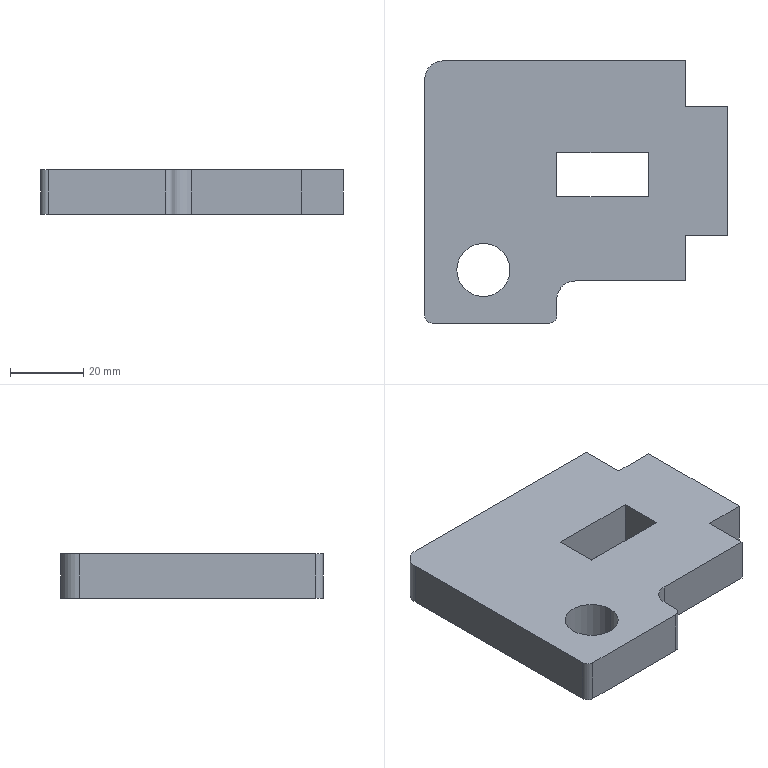Part | SolidWorks | features FlatPattern 1, SMBaseFlange 1, SheetMetal 1 | 1 solid | 22 faces | box 82.5 x 71.502 x 12 mm | volume 55316 mm3 | plane 16 | cylinder 6 | commonest cylinder face diameters 4 x2 10 x2 14.5 x2
STEP:
#1=CARTESIAN_POINT('',(-23.25,15.,12.));
#2=VERTEX_POINT('',#1);
#3=CARTESIAN_POINT('',(-8.75,15.,12.));
#4=VERTEX_POINT('',#3);
#5=CARTESIAN_POINT('',(-16.,15.,12.));
#6=DIRECTION('',(0.,0.,1.));
#7=DIRECTION('',(1.,0.,0.));
#8=AXIS2_PLACEMENT_3D('',#5,#6,#7);
#9=CIRCLE('',#8,7.25);
#10=EDGE_CURVE('',#2,#4,#9,.T.);
#11=ORIENTED_EDGE('',*,*,#10,.T.);
#12=CARTESIAN_POINT('',(-8.75,15.,0.));
#13=VERTEX_POINT('',#12);
#14=CARTESIAN_POINT('',(-8.75,15.,12.));
#15=DIRECTION('',(0.,0.,-1.));
#16=VECTOR('',#15,1000.);
#17=LINE('',#14,#16);
#18=EDGE_CURVE('',#4,#13,#17,.T.);
#19=ORIENTED_EDGE('',*,*,#18,.T.);
#20=CARTESIAN_POINT('',(-23.25,15.,0.));
#21=VERTEX_POINT('',#20);
#22=CARTESIAN_POINT('',(-16.,15.,0.));
#23=DIRECTION('',(0.,0.,1.));
#24=DIRECTION('',(1.,0.,0.));
#25=AXIS2_PLACEMENT_3D('',#22,#23,#24);
#26=CIRCLE('',#25,7.25);
#27=EDGE_CURVE('',#21,#13,#26,.T.);
#28=ORIENTED_EDGE('',*,*,#27,.F.);
#29=CARTESIAN_POINT('',(-23.25,15.,12.));
#30=DIRECTION('',(0.,0.,-1.));
#31=VECTOR('',#30,1000.);
#32=LINE('',#29,#31);
#33=EDGE_CURVE('',#2,#21,#32,.T.);
#34=ORIENTED_EDGE('',*,*,#33,.F.);
#35=EDGE_LOOP('',(#11,#19,#28,#34));
#36=FACE_OUTER_BOUND('',#35,.T.);
#37=CARTESIAN_POINT('',(-16.,15.,12.));
#38=DIRECTION('',(0.,0.,-1.));
#39=DIRECTION('',(-1.,0.,0.));
#40=AXIS2_PLACEMENT_3D('',#37,#38,#39);
#41=CYLINDRICAL_SURFACE('',#40,7.25);
#42=ADVANCED_FACE('',(#36),#41,.F.);
#43=CARTESIAN_POINT('',(39.,59.502,12.));
#44=VERTEX_POINT('',#43);
#45=CARTESIAN_POINT('',(39.,72.002,12.));
#46=VERTEX_POINT('',#45);
#47=CARTESIAN_POINT('',(39.,72.002,12.));
#48=DIRECTION('',(0.,1.,0.));
#49=VECTOR('',#48,1000.);
#50=LINE('',#47,#49);
#51=EDGE_CURVE('',#44,#46,#50,.T.);
#52=ORIENTED_EDGE('',*,*,#51,.T.);
#53=CARTESIAN_POINT('',(-27.,72.002,12.));
#54=VERTEX_POINT('',#53);
#55=CARTESIAN_POINT('',(-27.,72.002,12.));
#56=DIRECTION('',(-1.,0.,0.));
#57=VECTOR('',#56,1000.);
#58=LINE('',#55,#57);
#59=EDGE_CURVE('',#46,#54,#58,.T.);
#60=ORIENTED_EDGE('',*,*,#59,.T.);
#61=CARTESIAN_POINT('',(-32.,67.002,12.));
#62=VERTEX_POINT('',#61);
#63=CARTESIAN_POINT('',(-27.,67.002,12.));
#64=DIRECTION('',(0.,0.,1.));
#65=DIRECTION('',(-1.,0.,0.));
#66=AXIS2_PLACEMENT_3D('',#63,#64,#65);
#67=CIRCLE('',#66,5.);
#68=EDGE_CURVE('',#54,#62,#67,.T.);
#69=ORIENTED_EDGE('',*,*,#68,.T.);
#70=CARTESIAN_POINT('',(-32.,2.5,12.));
#71=VERTEX_POINT('',#70);
#72=CARTESIAN_POINT('',(-32.,2.5,12.));
#73=DIRECTION('',(0.,-1.,0.));
#74=VECTOR('',#73,1000.);
#75=LINE('',#72,#74);
#76=EDGE_CURVE('',#62,#71,#75,.T.);
#77=ORIENTED_EDGE('',*,*,#76,.T.);
#78=CARTESIAN_POINT('',(-30.,0.5,12.));
#79=VERTEX_POINT('',#78);
#80=CARTESIAN_POINT('',(-30.,2.5,12.));
#81=DIRECTION('',(0.,0.,1.));
#82=DIRECTION('',(-1.,0.,0.));
#83=AXIS2_PLACEMENT_3D('',#80,#81,#82);
#84=CIRCLE('',#83,2.);
#85=EDGE_CURVE('',#71,#79,#84,.T.);
#86=ORIENTED_EDGE('',*,*,#85,.T.);
#87=CARTESIAN_POINT('',(2.,0.5,12.));
#88=VERTEX_POINT('',#87);
#89=CARTESIAN_POINT('',(2.,0.5,12.));
#90=DIRECTION('',(1.,0.,0.));
#91=VECTOR('',#90,1000.);
#92=LINE('',#89,#91);
#93=EDGE_CURVE('',#79,#88,#92,.T.);
#94=ORIENTED_EDGE('',*,*,#93,.T.);
#95=CARTESIAN_POINT('',(4.,2.5,12.));
#96=VERTEX_POINT('',#95);
#97=CARTESIAN_POINT('',(2.,2.5,12.));
#98=DIRECTION('',(0.,0.,1.));
#99=DIRECTION('',(1.,0.,0.));
#100=AXIS2_PLACEMENT_3D('',#97,#98,#99);
#101=CIRCLE('',#100,2.);
#102=EDGE_CURVE('',#88,#96,#101,.T.);
#103=ORIENTED_EDGE('',*,*,#102,.T.);
#104=CARTESIAN_POINT('',(4.,7.002,12.));
#105=VERTEX_POINT('',#104);
#106=CARTESIAN_POINT('',(4.,7.002,12.));
#107=DIRECTION('',(0.,1.,0.));
#108=VECTOR('',#107,1000.);
#109=LINE('',#106,#108);
#110=EDGE_CURVE('',#96,#105,#109,.T.);
#111=ORIENTED_EDGE('',*,*,#110,.T.);
#112=CARTESIAN_POINT('',(9.,12.002,12.));
#113=VERTEX_POINT('',#112);
#114=CARTESIAN_POINT('',(9.,7.002,12.));
#115=DIRECTION('',(0.,0.,-1.));
#116=DIRECTION('',(1.,0.,0.));
#117=AXIS2_PLACEMENT_3D('',#114,#115,#116);
#118=CIRCLE('',#117,5.);
#119=EDGE_CURVE('',#105,#113,#118,.T.);
#120=ORIENTED_EDGE('',*,*,#119,.T.);
#121=CARTESIAN_POINT('',(39.,12.002,12.));
#122=VERTEX_POINT('',#121);
#123=CARTESIAN_POINT('',(39.,12.002,12.));
#124=DIRECTION('',(1.,0.,0.));
#125=VECTOR('',#124,1000.);
#126=LINE('',#123,#125);
#127=EDGE_CURVE('',#113,#122,#126,.T.);
#128=ORIENTED_EDGE('',*,*,#127,.T.);
#129=CARTESIAN_POINT('',(39.,24.502,12.));
#130=VERTEX_POINT('',#129);
#131=CARTESIAN_POINT('',(39.,24.502,12.));
#132=DIRECTION('',(0.,1.,0.));
#133=VECTOR('',#132,1000.);
#134=LINE('',#131,#133);
#135=EDGE_CURVE('',#122,#130,#134,.T.);
#136=ORIENTED_EDGE('',*,*,#135,.T.);
#137=CARTESIAN_POINT('',(50.5,24.502,12.));
#138=VERTEX_POINT('',#137);
#139=CARTESIAN_POINT('',(39.,24.502,12.));
#140=DIRECTION('',(1.,0.,0.));
#141=VECTOR('',#140,1000.);
#142=LINE('',#139,#141);
#143=EDGE_CURVE('',#130,#138,#142,.T.);
#144=ORIENTED_EDGE('',*,*,#143,.T.);
#145=CARTESIAN_POINT('',(50.5,59.502,12.));
#146=VERTEX_POINT('',#145);
#147=CARTESIAN_POINT('',(50.5,24.502,12.));
#148=DIRECTION('',(0.,1.,0.));
#149=VECTOR('',#148,1000.);
#150=LINE('',#147,#149);
#151=EDGE_CURVE('',#138,#146,#150,.T.);
#152=ORIENTED_EDGE('',*,*,#151,.T.);
#153=CARTESIAN_POINT('',(50.5,59.502,12.));
#154=DIRECTION('',(-1.,0.,0.));
#155=VECTOR('',#154,1000.);
#156=LINE('',#153,#155);
#157=EDGE_CURVE('',#146,#44,#156,.T.);
#158=ORIENTED_EDGE('',*,*,#157,.T.);
#159=EDGE_LOOP('',(#52,#60,#69,#77,#86,#94,#103,#111,#120,#128,#136,#144,#152,#158));
#160=FACE_OUTER_BOUND('',#159,.T.);
#161=ORIENTED_EDGE('',*,*,#10,.F.);
#162=CARTESIAN_POINT('',(-16.,15.,12.));
#163=DIRECTION('',(0.,0.,1.));
#164=DIRECTION('',(1.,0.,0.));
#165=AXIS2_PLACEMENT_3D('',#162,#163,#164);
#166=CIRCLE('',#165,7.25);
#167=EDGE_CURVE('',#4,#2,#166,.T.);
#168=ORIENTED_EDGE('',*,*,#167,.F.);
#169=EDGE_LOOP('',(#161,#168));
#170=FACE_BOUND('',#169,.T.);
#171=CARTESIAN_POINT('',(4.,35.002,12.));
#172=VERTEX_POINT('',#171);
#173=CARTESIAN_POINT('',(29.,35.002,12.));
#174=VERTEX_POINT('',#173);
#175=CARTESIAN_POINT('',(4.,35.002,12.));
#176=DIRECTION('',(1.,0.,0.));
#177=VECTOR('',#176,1000.);
#178=LINE('',#175,#177);
#179=EDGE_CURVE('',#172,#174,#178,.T.);
#180=ORIENTED_EDGE('',*,*,#179,.F.);
#181=CARTESIAN_POINT('',(4.,47.002,12.));
#182=VERTEX_POINT('',#181);
#183=CARTESIAN_POINT('',(4.,35.002,12.));
#184=DIRECTION('',(0.,-1.,0.));
#185=VECTOR('',#184,1000.);
#186=LINE('',#183,#185);
#187=EDGE_CURVE('',#182,#172,#186,.T.);
#188=ORIENTED_EDGE('',*,*,#187,.F.);
#189=CARTESIAN_POINT('',(29.,47.002,12.));
#190=VERTEX_POINT('',#189);
#191=CARTESIAN_POINT('',(4.,47.002,12.));
#192=DIRECTION('',(-1.,0.,0.));
#193=VECTOR('',#192,1000.);
#194=LINE('',#191,#193);
#195=EDGE_CURVE('',#190,#182,#194,.T.);
#196=ORIENTED_EDGE('',*,*,#195,.F.);
#197=CARTESIAN_POINT('',(29.,35.002,12.));
#198=DIRECTION('',(0.,1.,0.));
#199=VECTOR('',#198,1000.);
#200=LINE('',#197,#199);
#201=EDGE_CURVE('',#174,#190,#200,.T.);
#202=ORIENTED_EDGE('',*,*,#201,.F.);
#203=EDGE_LOOP('',(#180,#188,#196,#202));
#204=FACE_BOUND('',#203,.T.);
#205=CARTESIAN_POINT('',(9.,7.002,12.));
#206=DIRECTION('',(0.,0.,1.));
#207=DIRECTION('',(1.,0.,0.));
#208=AXIS2_PLACEMENT_3D('',#205,#206,#207);
#209=PLANE('',#208);
#210=ADVANCED_FACE('',(#160,#170,#204),#209,.T.);
#211=ORIENTED_EDGE('',*,*,#27,.T.);
#212=CARTESIAN_POINT('',(-16.,15.,0.));
#213=DIRECTION('',(0.,0.,1.));
#214=DIRECTION('',(1.,0.,0.));
#215=AXIS2_PLACEMENT_3D('',#212,#213,#214);
#216=CIRCLE('',#215,7.25);
#217=EDGE_CURVE('',#13,#21,#216,.T.);
#218=ORIENTED_EDGE('',*,*,#217,.T.);
#219=EDGE_LOOP('',(#211,#218));
#220=FACE_BOUND('',#219,.T.);
#221=CARTESIAN_POINT('',(39.,59.502,0.));
#222=VERTEX_POINT('',#221);
#223=CARTESIAN_POINT('',(39.,72.002,0.));
#224=VERTEX_POINT('',#223);
#225=CARTESIAN_POINT('',(39.,72.002,0.));
#226=DIRECTION('',(0.,1.,0.));
#227=VECTOR('',#226,1000.);
#228=LINE('',#225,#227);
#229=EDGE_CURVE('',#222,#224,#228,.T.);
#230=ORIENTED_EDGE('',*,*,#229,.F.);
#231=CARTESIAN_POINT('',(50.5,59.502,0.));
#232=VERTEX_POINT('',#231);
#233=CARTESIAN_POINT('',(50.5,59.502,0.));
#234=DIRECTION('',(-1.,0.,0.));
#235=VECTOR('',#234,1000.);
#236=LINE('',#233,#235);
#237=EDGE_CURVE('',#232,#222,#236,.T.);
#238=ORIENTED_EDGE('',*,*,#237,.F.);
#239=CARTESIAN_POINT('',(50.5,24.502,0.));
#240=VERTEX_POINT('',#239);
#241=CARTESIAN_POINT('',(50.5,24.502,0.));
#242=DIRECTION('',(0.,1.,0.));
#243=VECTOR('',#242,1000.);
#244=LINE('',#241,#243);
#245=EDGE_CURVE('',#240,#232,#244,.T.);
#246=ORIENTED_EDGE('',*,*,#245,.F.);
#247=CARTESIAN_POINT('',(39.,24.502,0.));
#248=VERTEX_POINT('',#247);
#249=CARTESIAN_POINT('',(39.,24.502,0.));
#250=DIRECTION('',(1.,0.,0.));
#251=VECTOR('',#250,1000.);
#252=LINE('',#249,#251);
#253=EDGE_CURVE('',#248,#240,#252,.T.);
#254=ORIENTED_EDGE('',*,*,#253,.F.);
#255=CARTESIAN_POINT('',(39.,12.002,0.));
#256=VERTEX_POINT('',#255);
#257=CARTESIAN_POINT('',(39.,24.502,0.));
#258=DIRECTION('',(0.,1.,0.));
#259=VECTOR('',#258,1000.);
#260=LINE('',#257,#259);
#261=EDGE_CURVE('',#256,#248,#260,.T.);
#262=ORIENTED_EDGE('',*,*,#261,.F.);
#263=CARTESIAN_POINT('',(9.,12.002,0.));
#264=VERTEX_POINT('',#263);
#265=CARTESIAN_POINT('',(39.,12.002,0.));
#266=DIRECTION('',(1.,0.,0.));
#267=VECTOR('',#266,1000.);
#268=LINE('',#265,#267);
#269=EDGE_CURVE('',#264,#256,#268,.T.);
#270=ORIENTED_EDGE('',*,*,#269,.F.);
#271=CARTESIAN_POINT('',(4.,7.002,0.));
#272=VERTEX_POINT('',#271);
#273=CARTESIAN_POINT('',(9.,7.002,0.));
#274=DIRECTION('',(0.,0.,-1.));
#275=DIRECTION('',(1.,0.,0.));
#276=AXIS2_PLACEMENT_3D('',#273,#274,#275);
#277=CIRCLE('',#276,5.);
#278=EDGE_CURVE('',#272,#264,#277,.T.);
#279=ORIENTED_EDGE('',*,*,#278,.F.);
#280=CARTESIAN_POINT('',(4.,2.5,0.));
#281=VERTEX_POINT('',#280);
#282=CARTESIAN_POINT('',(4.,7.002,0.));
#283=DIRECTION('',(0.,1.,0.));
#284=VECTOR('',#283,1000.);
#285=LINE('',#282,#284);
#286=EDGE_CURVE('',#281,#272,#285,.T.);
#287=ORIENTED_EDGE('',*,*,#286,.F.);
#288=CARTESIAN_POINT('',(2.,0.5,0.));
#289=VERTEX_POINT('',#288);
#290=CARTESIAN_POINT('',(2.,2.5,0.));
#291=DIRECTION('',(0.,0.,1.));
#292=DIRECTION('',(1.,0.,0.));
#293=AXIS2_PLACEMENT_3D('',#290,#291,#292);
#294=CIRCLE('',#293,2.);
#295=EDGE_CURVE('',#289,#281,#294,.T.);
#296=ORIENTED_EDGE('',*,*,#295,.F.);
#297=CARTESIAN_POINT('',(-30.,0.5,0.));
#298=VERTEX_POINT('',#297);
#299=CARTESIAN_POINT('',(2.,0.5,0.));
#300=DIRECTION('',(1.,0.,0.));
#301=VECTOR('',#300,1000.);
#302=LINE('',#299,#301);
#303=EDGE_CURVE('',#298,#289,#302,.T.);
#304=ORIENTED_EDGE('',*,*,#303,.F.);
#305=CARTESIAN_POINT('',(-32.,2.5,0.));
#306=VERTEX_POINT('',#305);
#307=CARTESIAN_POINT('',(-30.,2.5,0.));
#308=DIRECTION('',(0.,0.,1.));
#309=DIRECTION('',(-1.,0.,0.));
#310=AXIS2_PLACEMENT_3D('',#307,#308,#309);
#311=CIRCLE('',#310,2.);
#312=EDGE_CURVE('',#306,#298,#311,.T.);
#313=ORIENTED_EDGE('',*,*,#312,.F.);
#314=CARTESIAN_POINT('',(-32.,67.002,0.));
#315=VERTEX_POINT('',#314);
#316=CARTESIAN_POINT('',(-32.,2.5,0.));
#317=DIRECTION('',(0.,-1.,0.));
#318=VECTOR('',#317,1000.);
#319=LINE('',#316,#318);
#320=EDGE_CURVE('',#315,#306,#319,.T.);
#321=ORIENTED_EDGE('',*,*,#320,.F.);
#322=CARTESIAN_POINT('',(-27.,72.002,0.));
#323=VERTEX_POINT('',#322);
#324=CARTESIAN_POINT('',(-27.,67.002,0.));
#325=DIRECTION('',(0.,0.,1.));
#326=DIRECTION('',(-1.,0.,0.));
#327=AXIS2_PLACEMENT_3D('',#324,#325,#326);
#328=CIRCLE('',#327,5.);
#329=EDGE_CURVE('',#323,#315,#328,.T.);
#330=ORIENTED_EDGE('',*,*,#329,.F.);
#331=CARTESIAN_POINT('',(-27.,72.002,0.));
#332=DIRECTION('',(-1.,0.,0.));
#333=VECTOR('',#332,1000.);
#334=LINE('',#331,#333);
#335=EDGE_CURVE('',#224,#323,#334,.T.);
#336=ORIENTED_EDGE('',*,*,#335,.F.);
#337=EDGE_LOOP('',(#230,#238,#246,#254,#262,#270,#279,#287,#296,#304,#313,#321,#330,#336));
#338=FACE_OUTER_BOUND('',#337,.T.);
#339=CARTESIAN_POINT('',(4.,47.002,0.));
#340=VERTEX_POINT('',#339);
#341=CARTESIAN_POINT('',(4.,35.002,0.));
#342=VERTEX_POINT('',#341);
#343=CARTESIAN_POINT('',(4.,35.002,0.));
#344=DIRECTION('',(0.,-1.,0.));
#345=VECTOR('',#344,1000.);
#346=LINE('',#343,#345);
#347=EDGE_CURVE('',#340,#342,#346,.T.);
#348=ORIENTED_EDGE('',*,*,#347,.T.);
#349=CARTESIAN_POINT('',(29.,35.002,0.));
#350=VERTEX_POINT('',#349);
#351=CARTESIAN_POINT('',(4.,35.002,0.));
#352=DIRECTION('',(1.,0.,0.));
#353=VECTOR('',#352,1000.);
#354=LINE('',#351,#353);
#355=EDGE_CURVE('',#342,#350,#354,.T.);
#356=ORIENTED_EDGE('',*,*,#355,.T.);
#357=CARTESIAN_POINT('',(29.,47.002,0.));
#358=VERTEX_POINT('',#357);
#359=CARTESIAN_POINT('',(29.,35.002,0.));
#360=DIRECTION('',(0.,1.,0.));
#361=VECTOR('',#360,1000.);
#362=LINE('',#359,#361);
#363=EDGE_CURVE('',#350,#358,#362,.T.);
#364=ORIENTED_EDGE('',*,*,#363,.T.);
#365=CARTESIAN_POINT('',(4.,47.002,0.));
#366=DIRECTION('',(-1.,0.,0.));
#367=VECTOR('',#366,1000.);
#368=LINE('',#365,#367);
#369=EDGE_CURVE('',#358,#340,#368,.T.);
#370=ORIENTED_EDGE('',*,*,#369,.T.);
#371=EDGE_LOOP('',(#348,#356,#364,#370));
#372=FACE_BOUND('',#371,.T.);
#373=CARTESIAN_POINT('',(9.,7.002,0.));
#374=DIRECTION('',(0.,0.,1.));
#375=DIRECTION('',(1.,0.,0.));
#376=AXIS2_PLACEMENT_3D('',#373,#374,#375);
#377=PLANE('',#376);
#378=ADVANCED_FACE('',(#220,#338,#372),#377,.F.);
#379=ORIENTED_EDGE('',*,*,#229,.T.);
#380=CARTESIAN_POINT('',(39.,72.002,12.));
#381=DIRECTION('',(0.,0.,-1.));
#382=VECTOR('',#381,1000.);
#383=LINE('',#380,#382);
#384=EDGE_CURVE('',#46,#224,#383,.T.);
#385=ORIENTED_EDGE('',*,*,#384,.F.);
#386=ORIENTED_EDGE('',*,*,#51,.F.);
#387=CARTESIAN_POINT('',(39.,59.502,12.));
#388=DIRECTION('',(0.,0.,-1.));
#389=VECTOR('',#388,1000.);
#390=LINE('',#387,#389);
#391=EDGE_CURVE('',#44,#222,#390,.T.);
#392=ORIENTED_EDGE('',*,*,#391,.T.);
#393=EDGE_LOOP('',(#379,#385,#386,#392));
#394=FACE_OUTER_BOUND('',#393,.T.);
#395=CARTESIAN_POINT('',(39.,72.002,12.));
#396=DIRECTION('',(-1.,0.,0.));
#397=DIRECTION('',(0.,0.,1.));
#398=AXIS2_PLACEMENT_3D('',#395,#396,#397);
#399=PLANE('',#398);
#400=ADVANCED_FACE('',(#394),#399,.F.);
#401=ORIENTED_EDGE('',*,*,#335,.T.);
#402=CARTESIAN_POINT('',(-27.,72.002,12.));
#403=DIRECTION('',(0.,0.,-1.));
#404=VECTOR('',#403,1000.);
#405=LINE('',#402,#404);
#406=EDGE_CURVE('',#54,#323,#405,.T.);
#407=ORIENTED_EDGE('',*,*,#406,.F.);
#408=ORIENTED_EDGE('',*,*,#59,.F.);
#409=ORIENTED_EDGE('',*,*,#384,.T.);
#410=EDGE_LOOP('',(#401,#407,#408,#409));
#411=FACE_OUTER_BOUND('',#410,.T.);
#412=CARTESIAN_POINT('',(-27.,72.002,12.));
#413=DIRECTION('',(0.,-1.,0.));
#414=DIRECTION('',(0.,0.,-1.));
#415=AXIS2_PLACEMENT_3D('',#412,#413,#414);
#416=PLANE('',#415);
#417=ADVANCED_FACE('',(#411),#416,.F.);
#418=ORIENTED_EDGE('',*,*,#329,.T.);
#419=CARTESIAN_POINT('',(-32.,67.002,12.));
#420=DIRECTION('',(0.,0.,-1.));
#421=VECTOR('',#420,1000.);
#422=LINE('',#419,#421);
#423=EDGE_CURVE('',#62,#315,#422,.T.);
#424=ORIENTED_EDGE('',*,*,#423,.F.);
#425=ORIENTED_EDGE('',*,*,#68,.F.);
#426=ORIENTED_EDGE('',*,*,#406,.T.);
#427=EDGE_LOOP('',(#418,#424,#425,#426));
#428=FACE_OUTER_BOUND('',#427,.T.);
#429=CARTESIAN_POINT('',(-27.,67.002,12.));
#430=DIRECTION('',(0.,0.,-1.));
#431=DIRECTION('',(-1.,0.,0.));
#432=AXIS2_PLACEMENT_3D('',#429,#430,#431);
#433=CYLINDRICAL_SURFACE('',#432,5.);
#434=ADVANCED_FACE('',(#428),#433,.T.);
#435=ORIENTED_EDGE('',*,*,#320,.T.);
#436=CARTESIAN_POINT('',(-32.,2.5,12.));
#437=DIRECTION('',(0.,0.,-1.));
#438=VECTOR('',#437,1000.);
#439=LINE('',#436,#438);
#440=EDGE_CURVE('',#71,#306,#439,.T.);
#441=ORIENTED_EDGE('',*,*,#440,.F.);
#442=ORIENTED_EDGE('',*,*,#76,.F.);
#443=ORIENTED_EDGE('',*,*,#423,.T.);
#444=EDGE_LOOP('',(#435,#441,#442,#443));
#445=FACE_OUTER_BOUND('',#444,.T.);
#446=CARTESIAN_POINT('',(-32.,2.5,12.));
#447=DIRECTION('',(1.,0.,0.));
#448=DIRECTION('',(0.,1.,0.));
#449=AXIS2_PLACEMENT_3D('',#446,#447,#448);
#450=PLANE('',#449);
#451=ADVANCED_FACE('',(#445),#450,.F.);
#452=ORIENTED_EDGE('',*,*,#312,.T.);
#453=CARTESIAN_POINT('',(-30.,0.5,12.));
#454=DIRECTION('',(0.,0.,-1.));
#455=VECTOR('',#454,1000.);
#456=LINE('',#453,#455);
#457=EDGE_CURVE('',#79,#298,#456,.T.);
#458=ORIENTED_EDGE('',*,*,#457,.F.);
#459=ORIENTED_EDGE('',*,*,#85,.F.);
#460=ORIENTED_EDGE('',*,*,#440,.T.);
#461=EDGE_LOOP('',(#452,#458,#459,#460));
#462=FACE_OUTER_BOUND('',#461,.T.);
#463=CARTESIAN_POINT('',(-30.,2.5,12.));
#464=DIRECTION('',(0.,0.,-1.));
#465=DIRECTION('',(-1.,0.,0.));
#466=AXIS2_PLACEMENT_3D('',#463,#464,#465);
#467=CYLINDRICAL_SURFACE('',#466,2.);
#468=ADVANCED_FACE('',(#462),#467,.T.);
#469=ORIENTED_EDGE('',*,*,#303,.T.);
#470=CARTESIAN_POINT('',(2.,0.5,12.));
#471=DIRECTION('',(0.,0.,-1.));
#472=VECTOR('',#471,1000.);
#473=LINE('',#470,#472);
#474=EDGE_CURVE('',#88,#289,#473,.T.);
#475=ORIENTED_EDGE('',*,*,#474,.F.);
#476=ORIENTED_EDGE('',*,*,#93,.F.);
#477=ORIENTED_EDGE('',*,*,#457,.T.);
#478=EDGE_LOOP('',(#469,#475,#476,#477));
#479=FACE_OUTER_BOUND('',#478,.T.);
#480=CARTESIAN_POINT('',(2.,0.5,12.));
#481=DIRECTION('',(0.,1.,0.));
#482=DIRECTION('',(-1.,0.,0.));
#483=AXIS2_PLACEMENT_3D('',#480,#481,#482);
#484=PLANE('',#483);
#485=ADVANCED_FACE('',(#479),#484,.F.);
#486=ORIENTED_EDGE('',*,*,#295,.T.);
#487=CARTESIAN_POINT('',(4.,2.5,12.));
#488=DIRECTION('',(0.,0.,-1.));
#489=VECTOR('',#488,1000.);
#490=LINE('',#487,#489);
#491=EDGE_CURVE('',#96,#281,#490,.T.);
#492=ORIENTED_EDGE('',*,*,#491,.F.);
#493=ORIENTED_EDGE('',*,*,#102,.F.);
#494=ORIENTED_EDGE('',*,*,#474,.T.);
#495=EDGE_LOOP('',(#486,#492,#493,#494));
#496=FACE_OUTER_BOUND('',#495,.T.);
#497=CARTESIAN_POINT('',(2.,2.5,12.));
#498=DIRECTION('',(0.,0.,-1.));
#499=DIRECTION('',(-1.,0.,0.));
#500=AXIS2_PLACEMENT_3D('',#497,#498,#499);
#501=CYLINDRICAL_SURFACE('',#500,2.);
#502=ADVANCED_FACE('',(#496),#501,.T.);
#503=ORIENTED_EDGE('',*,*,#286,.T.);
#504=CARTESIAN_POINT('',(4.,7.002,12.));
#505=DIRECTION('',(0.,0.,-1.));
#506=VECTOR('',#505,1000.);
#507=LINE('',#504,#506);
#508=EDGE_CURVE('',#105,#272,#507,.T.);
#509=ORIENTED_EDGE('',*,*,#508,.F.);
#510=ORIENTED_EDGE('',*,*,#110,.F.);
#511=ORIENTED_EDGE('',*,*,#491,.T.);
#512=EDGE_LOOP('',(#503,#509,#510,#511));
#513=FACE_OUTER_BOUND('',#512,.T.);
#514=CARTESIAN_POINT('',(4.,7.002,12.));
#515=DIRECTION('',(-1.,0.,0.));
#516=DIRECTION('',(0.,0.,1.));
#517=AXIS2_PLACEMENT_3D('',#514,#515,#516);
#518=PLANE('',#517);
#519=ADVANCED_FACE('',(#513),#518,.F.);
#520=ORIENTED_EDGE('',*,*,#278,.T.);
#521=CARTESIAN_POINT('',(9.,12.002,12.));
#522=DIRECTION('',(0.,0.,-1.));
#523=VECTOR('',#522,1000.);
#524=LINE('',#521,#523);
#525=EDGE_CURVE('',#113,#264,#524,.T.);
#526=ORIENTED_EDGE('',*,*,#525,.F.);
#527=ORIENTED_EDGE('',*,*,#119,.F.);
#528=ORIENTED_EDGE('',*,*,#508,.T.);
#529=EDGE_LOOP('',(#520,#526,#527,#528));
#530=FACE_OUTER_BOUND('',#529,.T.);
#531=CARTESIAN_POINT('',(9.,7.002,12.));
#532=DIRECTION('',(0.,0.,-1.));
#533=DIRECTION('',(-1.,0.,0.));
#534=AXIS2_PLACEMENT_3D('',#531,#532,#533);
#535=CYLINDRICAL_SURFACE('',#534,5.);
#536=ADVANCED_FACE('',(#530),#535,.F.);
#537=ORIENTED_EDGE('',*,*,#269,.T.);
#538=CARTESIAN_POINT('',(39.,12.002,12.));
#539=DIRECTION('',(0.,0.,-1.));
#540=VECTOR('',#539,1000.);
#541=LINE('',#538,#540);
#542=EDGE_CURVE('',#122,#256,#541,.T.);
#543=ORIENTED_EDGE('',*,*,#542,.F.);
#544=ORIENTED_EDGE('',*,*,#127,.F.);
#545=ORIENTED_EDGE('',*,*,#525,.T.);
#546=EDGE_LOOP('',(#537,#543,#544,#545));
#547=FACE_OUTER_BOUND('',#546,.T.);
#548=CARTESIAN_POINT('',(39.,12.002,12.));
#549=DIRECTION('',(0.,1.,0.));
#550=DIRECTION('',(-1.,0.,0.));
#551=AXIS2_PLACEMENT_3D('',#548,#549,#550);
#552=PLANE('',#551);
#553=ADVANCED_FACE('',(#547),#552,.F.);
#554=ORIENTED_EDGE('',*,*,#261,.T.);
#555=CARTESIAN_POINT('',(39.,24.502,12.));
#556=DIRECTION('',(0.,0.,-1.));
#557=VECTOR('',#556,1000.);
#558=LINE('',#555,#557);
#559=EDGE_CURVE('',#130,#248,#558,.T.);
#560=ORIENTED_EDGE('',*,*,#559,.F.);
#561=ORIENTED_EDGE('',*,*,#135,.F.);
#562=ORIENTED_EDGE('',*,*,#542,.T.);
#563=EDGE_LOOP('',(#554,#560,#561,#562));
#564=FACE_OUTER_BOUND('',#563,.T.);
#565=CARTESIAN_POINT('',(39.,24.502,12.));
#566=DIRECTION('',(-1.,0.,0.));
#567=DIRECTION('',(0.,0.,1.));
#568=AXIS2_PLACEMENT_3D('',#565,#566,#567);
#569=PLANE('',#568);
#570=ADVANCED_FACE('',(#564),#569,.F.);
#571=ORIENTED_EDGE('',*,*,#253,.T.);
#572=CARTESIAN_POINT('',(50.5,24.502,12.));
#573=DIRECTION('',(0.,0.,-1.));
#574=VECTOR('',#573,1000.);
#575=LINE('',#572,#574);
#576=EDGE_CURVE('',#138,#240,#575,.T.);
#577=ORIENTED_EDGE('',*,*,#576,.F.);
#578=ORIENTED_EDGE('',*,*,#143,.F.);
#579=ORIENTED_EDGE('',*,*,#559,.T.);
#580=EDGE_LOOP('',(#571,#577,#578,#579));
#581=FACE_OUTER_BOUND('',#580,.T.);
#582=CARTESIAN_POINT('',(39.,24.502,12.));
#583=DIRECTION('',(0.,1.,0.));
#584=DIRECTION('',(0.,0.,1.));
#585=AXIS2_PLACEMENT_3D('',#582,#583,#584);
#586=PLANE('',#585);
#587=ADVANCED_FACE('',(#581),#586,.F.);
#588=ORIENTED_EDGE('',*,*,#245,.T.);
#589=CARTESIAN_POINT('',(50.5,59.502,12.));
#590=DIRECTION('',(0.,0.,-1.));
#591=VECTOR('',#590,1000.);
#592=LINE('',#589,#591);
#593=EDGE_CURVE('',#146,#232,#592,.T.);
#594=ORIENTED_EDGE('',*,*,#593,.F.);
#595=ORIENTED_EDGE('',*,*,#151,.F.);
#596=ORIENTED_EDGE('',*,*,#576,.T.);
#597=EDGE_LOOP('',(#588,#594,#595,#596));
#598=FACE_OUTER_BOUND('',#597,.T.);
#599=CARTESIAN_POINT('',(50.5,24.502,12.));
#600=DIRECTION('',(-1.,0.,0.));
#601=DIRECTION('',(0.,0.,1.));
#602=AXIS2_PLACEMENT_3D('',#599,#600,#601);
#603=PLANE('',#602);
#604=ADVANCED_FACE('',(#598),#603,.F.);
#605=ORIENTED_EDGE('',*,*,#237,.T.);
#606=ORIENTED_EDGE('',*,*,#391,.F.);
#607=ORIENTED_EDGE('',*,*,#157,.F.);
#608=ORIENTED_EDGE('',*,*,#593,.T.);
#609=EDGE_LOOP('',(#605,#606,#607,#608));
#610=FACE_OUTER_BOUND('',#609,.T.);
#611=CARTESIAN_POINT('',(50.5,59.502,12.));
#612=DIRECTION('',(0.,-1.,0.));
#613=DIRECTION('',(0.,0.,-1.));
#614=AXIS2_PLACEMENT_3D('',#611,#612,#613);
#615=PLANE('',#614);
#616=ADVANCED_FACE('',(#610),#615,.F.);
#617=ORIENTED_EDGE('',*,*,#18,.F.);
#618=ORIENTED_EDGE('',*,*,#167,.T.);
#619=ORIENTED_EDGE('',*,*,#33,.T.);
#620=ORIENTED_EDGE('',*,*,#217,.F.);
#621=EDGE_LOOP('',(#617,#618,#619,#620));
#622=FACE_OUTER_BOUND('',#621,.T.);
#623=CARTESIAN_POINT('',(-16.,15.,12.));
#624=DIRECTION('',(0.,0.,-1.));
#625=DIRECTION('',(-1.,0.,0.));
#626=AXIS2_PLACEMENT_3D('',#623,#624,#625);
#627=CYLINDRICAL_SURFACE('',#626,7.25);
#628=ADVANCED_FACE('',(#622),#627,.F.);
#629=ORIENTED_EDGE('',*,*,#347,.F.);
#630=CARTESIAN_POINT('',(4.,47.002,12.));
#631=DIRECTION('',(0.,0.,-1.));
#632=VECTOR('',#631,1000.);
#633=LINE('',#630,#632);
#634=EDGE_CURVE('',#182,#340,#633,.T.);
#635=ORIENTED_EDGE('',*,*,#634,.F.);
#636=ORIENTED_EDGE('',*,*,#187,.T.);
#637=CARTESIAN_POINT('',(4.,35.002,12.));
#638=DIRECTION('',(0.,0.,-1.));
#639=VECTOR('',#638,1000.);
#640=LINE('',#637,#639);
#641=EDGE_CURVE('',#172,#342,#640,.T.);
#642=ORIENTED_EDGE('',*,*,#641,.T.);
#643=EDGE_LOOP('',(#629,#635,#636,#642));
#644=FACE_OUTER_BOUND('',#643,.T.);
#645=CARTESIAN_POINT('',(4.,35.002,12.));
#646=DIRECTION('',(1.,0.,0.));
#647=DIRECTION('',(0.,0.,-1.));
#648=AXIS2_PLACEMENT_3D('',#645,#646,#647);
#649=PLANE('',#648);
#650=ADVANCED_FACE('',(#644),#649,.T.);
#651=ORIENTED_EDGE('',*,*,#355,.F.);
#652=ORIENTED_EDGE('',*,*,#641,.F.);
#653=ORIENTED_EDGE('',*,*,#179,.T.);
#654=CARTESIAN_POINT('',(29.,35.002,12.));
#655=DIRECTION('',(0.,0.,-1.));
#656=VECTOR('',#655,1000.);
#657=LINE('',#654,#656);
#658=EDGE_CURVE('',#174,#350,#657,.T.);
#659=ORIENTED_EDGE('',*,*,#658,.T.);
#660=EDGE_LOOP('',(#651,#652,#653,#659));
#661=FACE_OUTER_BOUND('',#660,.T.);
#662=CARTESIAN_POINT('',(4.,35.002,12.));
#663=DIRECTION('',(0.,1.,0.));
#664=DIRECTION('',(0.,0.,1.));
#665=AXIS2_PLACEMENT_3D('',#662,#663,#664);
#666=PLANE('',#665);
#667=ADVANCED_FACE('',(#661),#666,.T.);
#668=ORIENTED_EDGE('',*,*,#363,.F.);
#669=ORIENTED_EDGE('',*,*,#658,.F.);
#670=ORIENTED_EDGE('',*,*,#201,.T.);
#671=CARTESIAN_POINT('',(29.,47.002,12.));
#672=DIRECTION('',(0.,0.,-1.));
#673=VECTOR('',#672,1000.);
#674=LINE('',#671,#673);
#675=EDGE_CURVE('',#190,#358,#674,.T.);
#676=ORIENTED_EDGE('',*,*,#675,.T.);
#677=EDGE_LOOP('',(#668,#669,#670,#676));
#678=FACE_OUTER_BOUND('',#677,.T.);
#679=CARTESIAN_POINT('',(29.,35.002,12.));
#680=DIRECTION('',(-1.,0.,0.));
#681=DIRECTION('',(0.,0.,1.));
#682=AXIS2_PLACEMENT_3D('',#679,#680,#681);
#683=PLANE('',#682);
#684=ADVANCED_FACE('',(#678),#683,.T.);
#685=ORIENTED_EDGE('',*,*,#369,.F.);
#686=ORIENTED_EDGE('',*,*,#675,.F.);
#687=ORIENTED_EDGE('',*,*,#195,.T.);
#688=ORIENTED_EDGE('',*,*,#634,.T.);
#689=EDGE_LOOP('',(#685,#686,#687,#688));
#690=FACE_OUTER_BOUND('',#689,.T.);
#691=CARTESIAN_POINT('',(4.,47.002,12.));
#692=DIRECTION('',(0.,-1.,0.));
#693=DIRECTION('',(0.,0.,-1.));
#694=AXIS2_PLACEMENT_3D('',#691,#692,#693);
#695=PLANE('',#694);
#696=ADVANCED_FACE('',(#690),#695,.T.);
#697=CLOSED_SHELL('',(#42,#210,#378,#400,#417,#434,#451,#468,#485,#502,#519,#536,#553,#570,#587,#604,#616,#628,#650,#667,#684,#696));
#698=MANIFOLD_SOLID_BREP('',#697);
#699=CARTESIAN_POINT('',(0.,0.,0.));
#700=DIRECTION('',(0.,0.,1.));
#701=DIRECTION('',(1.,0.,0.));
#702=AXIS2_PLACEMENT_3D('',#699,#700,#701);
#703=(LENGTH_UNIT()NAMED_UNIT(*)SI_UNIT(.MILLI.,.METRE.));
#704=UNCERTAINTY_MEASURE_WITH_UNIT(LENGTH_MEASURE(0.00001),#703,'','');
#705=(NAMED_UNIT(*)PLANE_ANGLE_UNIT()SI_UNIT($,.RADIAN.));
#706=(NAMED_UNIT(*)SI_UNIT($,.STERADIAN.)SOLID_ANGLE_UNIT());
#707=(GEOMETRIC_REPRESENTATION_CONTEXT(3)GLOBAL_UNCERTAINTY_ASSIGNED_CONTEXT((#704))GLOBAL_UNIT_ASSIGNED_CONTEXT((#703,#705,#706))REPRESENTATION_CONTEXT('',''));
#708=ADVANCED_BREP_SHAPE_REPRESENTATION('',(#698,#702),#707);